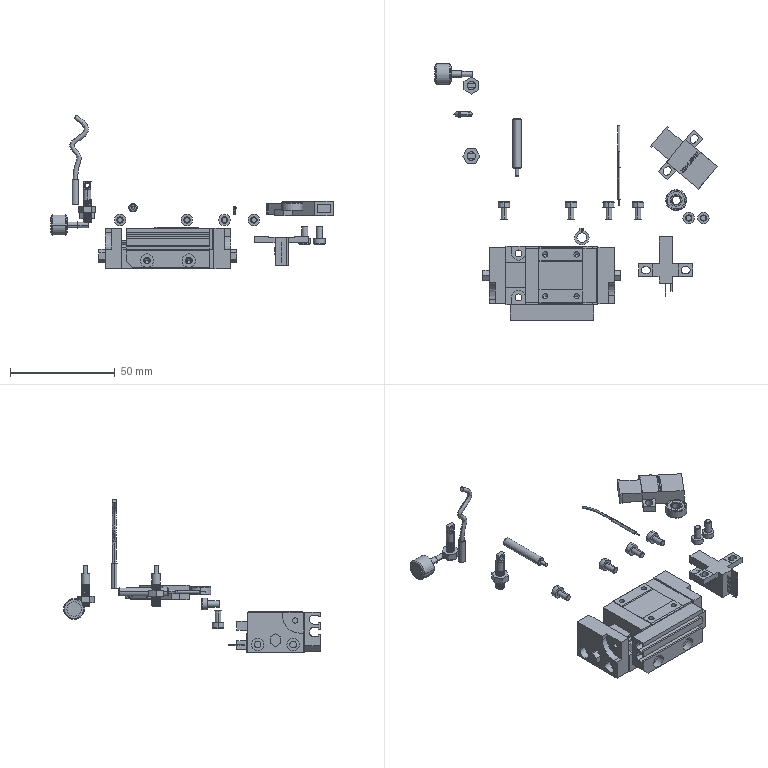Part | NX | 23 solids | 1567 faces | box 135.115 x 122.7 x 73.598 mm | volume 39087 mm3 | plane 1221 | cylinder 232 | cone 84 | spline 18 | torus 11 | sphere 1 | commonest cylinder face diameters 4 x62 2.5 x30 3.2 x24 3 x20 3.3 x12 5.5 x12